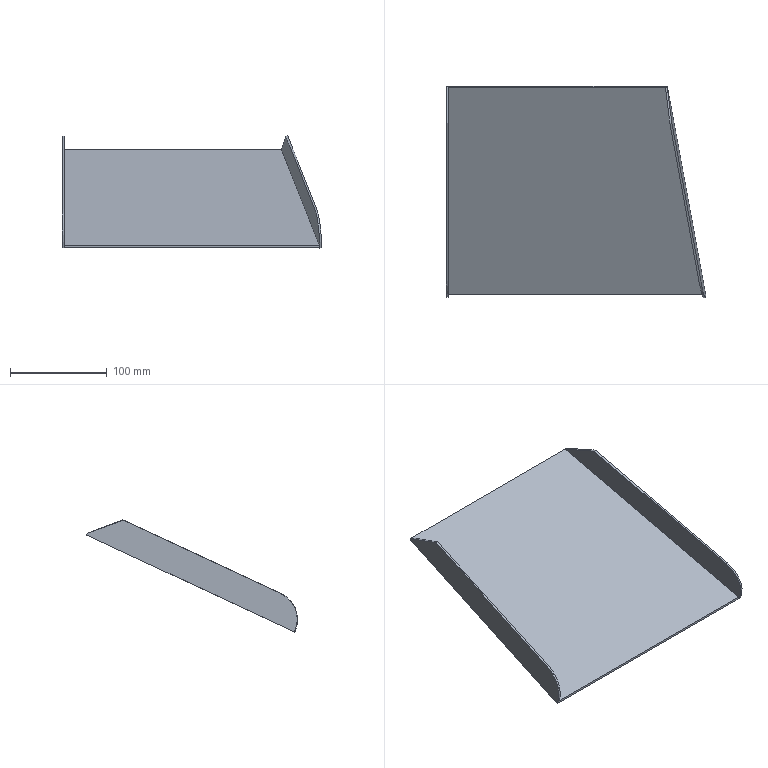Part | NX | features solid 2 | 1 solid | 14 faces | box 267.814 x 218.199 x 115.938 mm | volume 140586 mm3 | plane 11 | cylinder 2 | spline 1 | commonest cylinder face diameters 60 x2
STEP:
#1=CARTESIAN_POINT('',(712.,-840.,-299.582));
#2=VERTEX_POINT('',#1);
#3=CARTESIAN_POINT('',(975.787,-840.,-299.582));
#4=VERTEX_POINT('',#3);
#5=CARTESIAN_POINT('',(-476.248,-840.,-299.582));
#6=DIRECTION('',(1.,0.,0.));
#7=VECTOR('',#6,1000.);
#8=LINE('',#5,#7);
#9=EDGE_CURVE('',#2,#4,#8,.T.);
#10=ORIENTED_EDGE('',*,*,#9,.T.);
#11=CARTESIAN_POINT('',(975.631,-840.,-297.376));
#12=VERTEX_POINT('',#11);
#13=CARTESIAN_POINT('',(998.098,-840.,-616.062));
#14=DIRECTION('',(-0.07032,0.,0.9975));
#15=VECTOR('',#14,1000.);
#16=LINE('',#13,#15);
#17=EDGE_CURVE('',#4,#12,#16,.T.);
#18=ORIENTED_EDGE('',*,*,#17,.T.);
#19=CARTESIAN_POINT('',(712.,-840.,-297.376));
#20=VERTEX_POINT('',#19);
#21=CARTESIAN_POINT('',(-476.248,-840.,-297.376));
#22=DIRECTION('',(1.,0.,0.));
#23=VECTOR('',#22,1000.);
#24=LINE('',#21,#23);
#25=EDGE_CURVE('',#20,#12,#24,.T.);
#26=ORIENTED_EDGE('',*,*,#25,.F.);
#27=CARTESIAN_POINT('',(712.,-840.,-720.));
#28=DIRECTION('',(0.,0.,1.));
#29=VECTOR('',#28,1000.);
#30=LINE('',#27,#29);
#31=EDGE_CURVE('',#2,#20,#30,.T.);
#32=ORIENTED_EDGE('',*,*,#31,.F.);
#33=EDGE_LOOP('',(#10,#18,#26,#32));
#34=FACE_BOUND('',#33,.T.);
#35=CARTESIAN_POINT('',(-476.248,-840.,-720.));
#36=DIRECTION('',(0.,1.,0.));
#37=DIRECTION('',(-1.,0.,0.));
#38=AXIS2_PLACEMENT_3D('',#35,#36,#37);
#39=PLANE('',#38);
#40=ADVANCED_FACE('',(#34),#39,.F.);
#41=CARTESIAN_POINT('',(936.259,-626.089,-197.627));
#42=VERTEX_POINT('',#41);
#43=CARTESIAN_POINT('',(882.666,-334.91,-61.848));
#44=DIRECTION('',(0.1645,-0.894,-0.4169));
#45=VECTOR('',#44,1000.);
#46=LINE('',#43,#45);
#47=EDGE_CURVE('',#42,#12,#46,.T.);
#48=ORIENTED_EDGE('',*,*,#47,.F.);
#49=CARTESIAN_POINT('',(938.232,-625.791,-197.488));
#50=VERTEX_POINT('',#49);
#51=CARTESIAN_POINT('',(938.232,-625.791,-197.488));
#52=DIRECTION('',(0.9864,0.1491,0.06954));
#53=VECTOR('',#52,1000.);
#54=LINE('',#51,#53);
#55=EDGE_CURVE('',#42,#50,#54,.T.);
#56=ORIENTED_EDGE('',*,*,#55,.T.);
#57=CARTESIAN_POINT('',(712.,-626.036,-197.603));
#58=VERTEX_POINT('',#57);
#59=CARTESIAN_POINT('',(938.232,-625.791,-197.488));
#60=CARTESIAN_POINT('',(937.864,-625.821,-197.502));
#61=CARTESIAN_POINT('',(937.156,-625.853,-197.517));
#62=CARTESIAN_POINT('',(936.019,-625.866,-197.523));
#63=CARTESIAN_POINT('',(935.325,-625.866,-197.523));
#64=CARTESIAN_POINT('',(934.661,-625.862,-197.521));
#65=CARTESIAN_POINT('',(934.351,-625.859,-197.52));
#66=CARTESIAN_POINT('',(933.814,-625.856,-197.518));
#67=CARTESIAN_POINT('',(933.119,-625.851,-197.516));
#68=CARTESIAN_POINT('',(932.217,-625.847,-197.514));
#69=CARTESIAN_POINT('',(931.124,-625.843,-197.513));
#70=CARTESIAN_POINT('',(930.365,-625.841,-197.512));
#71=CARTESIAN_POINT('',(929.239,-625.839,-197.511));
#72=CARTESIAN_POINT('',(927.81,-625.837,-197.51));
#73=CARTESIAN_POINT('',(926.307,-625.836,-197.509));
#74=CARTESIAN_POINT('',(925.211,-625.836,-197.509));
#75=CARTESIAN_POINT('',(924.592,-625.836,-197.509));
#76=CARTESIAN_POINT('',(923.901,-625.836,-197.509));
#77=CARTESIAN_POINT('',(923.486,-625.836,-197.509));
#78=CARTESIAN_POINT('',(922.62,-625.837,-197.51));
#79=CARTESIAN_POINT('',(921.494,-625.838,-197.51));
#80=CARTESIAN_POINT('',(919.967,-625.841,-197.511));
#81=CARTESIAN_POINT('',(918.293,-625.844,-197.513));
#82=CARTESIAN_POINT('',(916.464,-625.847,-197.515));
#83=CARTESIAN_POINT('',(914.484,-625.852,-197.517));
#84=CARTESIAN_POINT('',(912.698,-625.856,-197.519));
#85=CARTESIAN_POINT('',(911.212,-625.86,-197.52));
#86=CARTESIAN_POINT('',(910.306,-625.862,-197.521));
#87=CARTESIAN_POINT('',(909.757,-625.864,-197.522));
#88=CARTESIAN_POINT('',(909.228,-625.865,-197.523));
#89=CARTESIAN_POINT('',(908.354,-625.867,-197.524));
#90=CARTESIAN_POINT('',(906.61,-625.872,-197.526));
#91=CARTESIAN_POINT('',(904.237,-625.878,-197.529));
#92=CARTESIAN_POINT('',(901.543,-625.885,-197.532));
#93=CARTESIAN_POINT('',(898.171,-625.894,-197.536));
#94=CARTESIAN_POINT('',(894.359,-625.903,-197.541));
#95=CARTESIAN_POINT('',(890.432,-625.913,-197.545));
#96=CARTESIAN_POINT('',(887.154,-625.921,-197.549));
#97=CARTESIAN_POINT('',(884.521,-625.928,-197.552));
#98=CARTESIAN_POINT('',(882.871,-625.932,-197.554));
#99=CARTESIAN_POINT('',(881.991,-625.933,-197.555));
#100=CARTESIAN_POINT('',(881.583,-625.934,-197.555));
#101=CARTESIAN_POINT('',(881.33,-625.935,-197.555));
#102=CARTESIAN_POINT('',(881.219,-625.935,-197.555));
#103=CARTESIAN_POINT('',(880.86,-625.936,-197.556));
#104=CARTESIAN_POINT('',(880.282,-625.937,-197.556));
#105=CARTESIAN_POINT('',(879.042,-625.939,-197.557));
#106=CARTESIAN_POINT('',(876.424,-625.942,-197.559));
#107=CARTESIAN_POINT('',(872.189,-625.947,-197.561));
#108=CARTESIAN_POINT('',(866.348,-625.953,-197.564));
#109=CARTESIAN_POINT('',(859.739,-625.957,-197.566));
#110=CARTESIAN_POINT('',(852.364,-625.961,-197.568));
#111=CARTESIAN_POINT('',(845.58,-625.964,-197.569));
#112=CARTESIAN_POINT('',(839.769,-625.966,-197.57));
#113=CARTESIAN_POINT('',(835.221,-625.967,-197.57));
#114=CARTESIAN_POINT('',(831.267,-625.968,-197.571));
#115=CARTESIAN_POINT('',(828.017,-625.969,-197.571));
#116=CARTESIAN_POINT('',(826.135,-625.969,-197.571));
#117=CARTESIAN_POINT('',(824.894,-625.969,-197.571));
#118=CARTESIAN_POINT('',(823.993,-625.97,-197.571));
#119=CARTESIAN_POINT('',(823.37,-625.97,-197.572));
#120=CARTESIAN_POINT('',(822.475,-625.97,-197.572));
#121=CARTESIAN_POINT('',(820.761,-625.97,-197.572));
#122=CARTESIAN_POINT('',(817.,-625.971,-197.572));
#123=CARTESIAN_POINT('',(811.23,-625.972,-197.573));
#124=CARTESIAN_POINT('',(804.273,-625.974,-197.574));
#125=CARTESIAN_POINT('',(794.975,-625.977,-197.575));
#126=CARTESIAN_POINT('',(783.298,-625.982,-197.577));
#127=CARTESIAN_POINT('',(769.206,-625.99,-197.581));
#128=CARTESIAN_POINT('',(755.031,-625.999,-197.585));
#129=CARTESIAN_POINT('',(736.021,-626.013,-197.592));
#130=CARTESIAN_POINT('',(721.641,-626.026,-197.598));
#131=CARTESIAN_POINT('',(712.,-626.036,-197.603));
#132=B_SPLINE_CURVE_WITH_KNOTS('',3,(#59,#60,#61,#62,#63,#64,#65,#66,#67,#68,#69,#70,#71,#72,#73,#74,#75,#76,#77,#78,#79,#80,#81,#82,#83,#84,#85,#86,#87,#88,#89,#90,#91,#92,#93,#94,#95,#96,#97,#98,#99,#100,#101,#102,#103,#104,#105,#106,#107,#108,#109,#110,#111,#112,#113,#114,#115,#116,#117,#118,#119,#120,#121,#122,#123,#124,#125,#126,#127,#128,#129,#130,#131),.UNSPECIFIED.,.F.,.F.,(4,1,1,1,1,1,1,1,1,1,1,1,1,1,1,1,1,1,1,1,1,1,1,1,1,1,1,1,1,1,1,1,1,1,1,1,1,1,1,1,1,1,1,1,1,1,1,1,1,1,1,1,1,1,1,1,1,1,1,1,1,1,1,1,1,1,1,1,1,1,4),(0.,0.007746,0.01162,0.01355,0.01549,0.01743,0.01936,0.02324,0.02711,0.03098,0.03486,0.03873,0.04647,0.05422,0.05809,0.06003,0.06196,0.06584,0.06971,0.07746,0.0852,0.09295,0.1007,0.1084,0.1162,0.1201,0.1239,0.1249,0.1259,0.1278,0.1317,0.1394,0.1472,0.1549,0.1704,0.1859,0.2014,0.2169,0.2324,0.2401,0.244,0.2479,0.2498,0.2517,0.2556,0.2633,0.2788,0.3098,0.3408,0.3718,0.4028,0.4338,0.4492,0.4647,0.4802,0.488,0.4957,0.4977,0.4996,0.5035,0.5073,0.5112,0.5267,0.5577,0.5887,0.6196,0.6816,0.7436,0.8055,0.8675,0.9914),.UNSPECIFIED.);
#133=EDGE_CURVE('',#58,#50,#132,.F.);
#134=ORIENTED_EDGE('',*,*,#133,.F.);
#135=CARTESIAN_POINT('',(712.,-651.161,-209.318));
#136=DIRECTION('',(0.,-0.9063,-0.4226));
#137=VECTOR('',#136,1000.);
#138=LINE('',#135,#137);
#139=EDGE_CURVE('',#58,#20,#138,.T.);
#140=ORIENTED_EDGE('',*,*,#139,.T.);
#141=ORIENTED_EDGE('',*,*,#25,.T.);
#142=EDGE_LOOP('',(#48,#56,#134,#140,#141));
#143=FACE_BOUND('',#142,.T.);
#144=CARTESIAN_POINT('',(-1209.175,-651.161,-209.318));
#145=DIRECTION('',(0.,-0.4226,0.9063));
#146=DIRECTION('',(1.,0.,0.));
#147=AXIS2_PLACEMENT_3D('',#144,#145,#146);
#148=PLANE('',#147);
#149=ADVANCED_FACE('',(#143),#148,.T.);
#150=CARTESIAN_POINT('',(972.878,-825.86,-259.887));
#151=VERTEX_POINT('',#150);
#152=CARTESIAN_POINT('',(977.814,-840.,-299.582));
#153=VERTEX_POINT('',#152);
#154=CARTESIAN_POINT('',(972.878,-813.181,-287.077));
#155=DIRECTION('',(-0.9864,-0.1491,-0.06954));
#156=DIRECTION('',(0.1495,-0.9888,0.));
#157=AXIS2_PLACEMENT_3D('',#154,#155,#156);
#158=CIRCLE('',#157,30.);
#159=EDGE_CURVE('',#151,#153,#158,.F.);
#160=ORIENTED_EDGE('',*,*,#159,.T.);
#161=CARTESIAN_POINT('',(938.232,-624.945,-199.301));
#162=VERTEX_POINT('',#161);
#163=CARTESIAN_POINT('',(884.639,-333.767,-63.522));
#164=DIRECTION('',(0.1645,-0.894,-0.4169));
#165=VECTOR('',#164,1000.);
#166=LINE('',#163,#165);
#167=EDGE_CURVE('',#162,#153,#166,.T.);
#168=ORIENTED_EDGE('',*,*,#167,.F.);
#169=CARTESIAN_POINT('',(938.232,-624.945,-199.301));
#170=CARTESIAN_POINT('',(938.232,-625.227,-198.696));
#171=CARTESIAN_POINT('',(938.232,-625.509,-198.092));
#172=CARTESIAN_POINT('',(938.232,-625.791,-197.488));
#173=B_SPLINE_CURVE_WITH_KNOTS('',3,(#169,#170,#171,#172),.UNSPECIFIED.,.F.,.F.,(4,4),(0.,1.),.UNSPECIFIED.);
#174=EDGE_CURVE('',#50,#162,#173,.F.);
#175=ORIENTED_EDGE('',*,*,#174,.F.);
#176=CARTESIAN_POINT('',(942.839,-662.655,-183.783));
#177=VERTEX_POINT('',#176);
#178=CARTESIAN_POINT('',(942.839,-662.655,-183.783));
#179=DIRECTION('',(-0.1163,0.931,-0.3461));
#180=VECTOR('',#179,1000.);
#181=LINE('',#178,#180);
#182=EDGE_CURVE('',#50,#177,#181,.F.);
#183=ORIENTED_EDGE('',*,*,#182,.T.);
#184=CARTESIAN_POINT('',(938.232,-637.624,-172.111));
#185=DIRECTION('',(0.1645,-0.894,-0.4169));
#186=VECTOR('',#185,1000.);
#187=LINE('',#184,#186);
#188=EDGE_CURVE('',#177,#151,#187,.T.);
#189=ORIENTED_EDGE('',*,*,#188,.T.);
#190=EDGE_LOOP('',(#160,#168,#175,#183,#189));
#191=FACE_BOUND('',#190,.T.);
#192=CARTESIAN_POINT('',(884.639,-334.612,-61.709));
#193=DIRECTION('',(0.9864,0.1491,0.06954));
#194=DIRECTION('',(-0.1495,0.9888,0.));
#195=AXIS2_PLACEMENT_3D('',#192,#193,#194);
#196=PLANE('',#195);
#197=ADVANCED_FACE('',(#191),#196,.T.);
#198=CARTESIAN_POINT('',(710.,-625.193,-199.416));
#199=VERTEX_POINT('',#198);
#200=CARTESIAN_POINT('',(938.232,-624.945,-199.301));
#201=CARTESIAN_POINT('',(937.861,-624.976,-199.315));
#202=CARTESIAN_POINT('',(937.146,-625.008,-199.33));
#203=CARTESIAN_POINT('',(935.994,-625.021,-199.336));
#204=CARTESIAN_POINT('',(935.293,-625.021,-199.336));
#205=CARTESIAN_POINT('',(934.612,-625.017,-199.334));
#206=CARTESIAN_POINT('',(934.327,-625.014,-199.333));
#207=CARTESIAN_POINT('',(933.775,-625.01,-199.331));
#208=CARTESIAN_POINT('',(933.074,-625.006,-199.329));
#209=CARTESIAN_POINT('',(932.161,-625.002,-199.327));
#210=CARTESIAN_POINT('',(931.043,-624.998,-199.325));
#211=CARTESIAN_POINT('',(930.308,-624.996,-199.324));
#212=CARTESIAN_POINT('',(929.159,-624.994,-199.323));
#213=CARTESIAN_POINT('',(928.01,-624.992,-199.322));
#214=CARTESIAN_POINT('',(926.804,-624.991,-199.322));
#215=CARTESIAN_POINT('',(925.885,-624.99,-199.322));
#216=CARTESIAN_POINT('',(925.087,-624.99,-199.322));
#217=CARTESIAN_POINT('',(924.471,-624.991,-199.322));
#218=CARTESIAN_POINT('',(923.915,-624.991,-199.322));
#219=CARTESIAN_POINT('',(923.692,-624.991,-199.322));
#220=CARTESIAN_POINT('',(923.263,-624.991,-199.322));
#221=CARTESIAN_POINT('',(922.533,-624.992,-199.322));
#222=CARTESIAN_POINT('',(921.363,-624.993,-199.323));
#223=CARTESIAN_POINT('',(919.816,-624.996,-199.324));
#224=CARTESIAN_POINT('',(918.111,-624.999,-199.326));
#225=CARTESIAN_POINT('',(916.249,-625.003,-199.327));
#226=CARTESIAN_POINT('',(914.234,-625.007,-199.33));
#227=CARTESIAN_POINT('',(912.417,-625.012,-199.332));
#228=CARTESIAN_POINT('',(911.093,-625.015,-199.333));
#229=CARTESIAN_POINT('',(910.291,-625.017,-199.334));
#230=CARTESIAN_POINT('',(909.755,-625.018,-199.335));
#231=CARTESIAN_POINT('',(908.92,-625.021,-199.336));
#232=CARTESIAN_POINT('',(907.928,-625.023,-199.337));
#233=CARTESIAN_POINT('',(906.178,-625.028,-199.339));
#234=CARTESIAN_POINT('',(903.808,-625.034,-199.342));
#235=CARTESIAN_POINT('',(901.116,-625.041,-199.345));
#236=CARTESIAN_POINT('',(897.752,-625.049,-199.349));
#237=CARTESIAN_POINT('',(893.956,-625.059,-199.354));
#238=CARTESIAN_POINT('',(890.061,-625.069,-199.358));
#239=CARTESIAN_POINT('',(886.824,-625.077,-199.362));
#240=CARTESIAN_POINT('',(884.675,-625.082,-199.364));
#241=CARTESIAN_POINT('',(883.287,-625.085,-199.366));
#242=CARTESIAN_POINT('',(882.405,-625.087,-199.367));
#243=CARTESIAN_POINT('',(881.827,-625.089,-199.367));
#244=CARTESIAN_POINT('',(881.401,-625.089,-199.368));
#245=CARTESIAN_POINT('',(881.251,-625.09,-199.368));
#246=CARTESIAN_POINT('',(880.651,-625.091,-199.368));
#247=CARTESIAN_POINT('',(879.987,-625.092,-199.369));
#248=CARTESIAN_POINT('',(878.713,-625.094,-199.37));
#249=CARTESIAN_POINT('',(876.807,-625.096,-199.371));
#250=CARTESIAN_POINT('',(874.309,-625.1,-199.373));
#251=CARTESIAN_POINT('',(870.725,-625.103,-199.374));
#252=CARTESIAN_POINT('',(865.755,-625.108,-199.376));
#253=CARTESIAN_POINT('',(859.012,-625.113,-199.379));
#254=CARTESIAN_POINT('',(851.49,-625.117,-199.381));
#255=CARTESIAN_POINT('',(844.572,-625.119,-199.382));
#256=CARTESIAN_POINT('',(838.648,-625.121,-199.383));
#257=CARTESIAN_POINT('',(834.783,-625.122,-199.383));
#258=CARTESIAN_POINT('',(831.594,-625.123,-199.383));
#259=CARTESIAN_POINT('',(829.151,-625.123,-199.384));
#260=CARTESIAN_POINT('',(827.085,-625.124,-199.384));
#261=CARTESIAN_POINT('',(825.596,-625.124,-199.384));
#262=CARTESIAN_POINT('',(824.772,-625.124,-199.384));
#263=CARTESIAN_POINT('',(824.058,-625.124,-199.384));
#264=CARTESIAN_POINT('',(823.697,-625.124,-199.384));
#265=CARTESIAN_POINT('',(823.092,-625.124,-199.384));
#266=CARTESIAN_POINT('',(822.091,-625.125,-199.384));
#267=CARTESIAN_POINT('',(820.63,-625.125,-199.384));
#268=CARTESIAN_POINT('',(818.888,-625.125,-199.385));
#269=CARTESIAN_POINT('',(816.559,-625.126,-199.385));
#270=CARTESIAN_POINT('',(813.647,-625.126,-199.385));
#271=CARTESIAN_POINT('',(808.978,-625.127,-199.386));
#272=CARTESIAN_POINT('',(803.13,-625.129,-199.386));
#273=CARTESIAN_POINT('',(796.092,-625.132,-199.388));
#274=CARTESIAN_POINT('',(789.033,-625.135,-199.389));
#275=CARTESIAN_POINT('',(779.592,-625.139,-199.391));
#276=CARTESIAN_POINT('',(767.74,-625.146,-199.394));
#277=CARTESIAN_POINT('',(753.434,-625.155,-199.398));
#278=CARTESIAN_POINT('',(734.247,-625.17,-199.405));
#279=CARTESIAN_POINT('',(719.732,-625.183,-199.412));
#280=CARTESIAN_POINT('',(710.,-625.193,-199.416));
#281=B_SPLINE_CURVE_WITH_KNOTS('',3,(#200,#201,#202,#203,#204,#205,#206,#207,#208,#209,#210,#211,#212,#213,#214,#215,#216,#217,#218,#219,#220,#221,#222,#223,#224,#225,#226,#227,#228,#229,#230,#231,#232,#233,#234,#235,#236,#237,#238,#239,#240,#241,#242,#243,#244,#245,#246,#247,#248,#249,#250,#251,#252,#253,#254,#255,#256,#257,#258,#259,#260,#261,#262,#263,#264,#265,#266,#267,#268,#269,#270,#271,#272,#273,#274,#275,#276,#277,#278,#279,#280),.UNSPECIFIED.,.F.,.F.,(4,1,1,1,1,1,1,1,1,1,1,1,1,1,1,1,1,1,1,1,1,1,1,1,1,1,1,1,1,1,1,1,1,1,1,1,1,1,1,1,1,1,1,1,1,1,1,1,1,1,1,1,1,1,1,1,1,1,1,1,1,1,1,1,1,1,1,1,1,1,1,1,1,1,1,1,1,1,4),(0.,0.007812,0.01172,0.01367,0.01562,0.01758,0.01953,0.02344,0.02734,0.03125,0.03516,0.03906,0.04688,0.05078,0.05469,0.05859,0.06055,0.0625,0.06445,0.06641,0.07031,0.07812,0.08594,0.09375,0.1016,0.1094,0.1172,0.1211,0.123,0.125,0.127,0.1289,0.1328,0.1406,0.1484,0.1562,0.1719,0.1875,0.2031,0.2188,0.2266,0.2344,0.2422,0.2461,0.25,0.2539,0.2578,0.2656,0.2812,0.2969,0.3125,0.3438,0.375,0.4062,0.4375,0.4531,0.4688,0.4766,0.4844,0.4922,0.4961,0.498,0.5,0.502,0.5039,0.5078,0.5156,0.5234,0.5312,0.5469,0.5625,0.5938,0.625,0.6562,0.6875,0.75,0.8125,0.875,1.),.UNSPECIFIED.);
#282=EDGE_CURVE('',#199,#162,#281,.F.);
#283=ORIENTED_EDGE('',*,*,#282,.F.);
#284=CARTESIAN_POINT('',(710.,-626.038,-197.604));
#285=VERTEX_POINT('',#284);
#286=CARTESIAN_POINT('',(710.,-626.038,-197.604));
#287=CARTESIAN_POINT('',(710.,-625.757,-198.208));
#288=CARTESIAN_POINT('',(710.,-625.475,-198.812));
#289=CARTESIAN_POINT('',(710.,-625.193,-199.416));
#290=B_SPLINE_CURVE_WITH_KNOTS('',3,(#286,#287,#288,#289),.UNSPECIFIED.,.F.,.F.,(4,4),(0.,1.),.UNSPECIFIED.);
#291=EDGE_CURVE('',#285,#199,#290,.T.);
#292=ORIENTED_EDGE('',*,*,#291,.F.);
#293=CARTESIAN_POINT('',(712.,-626.038,-197.604));
#294=CARTESIAN_POINT('',(711.333,-626.038,-197.604));
#295=CARTESIAN_POINT('',(710.667,-626.038,-197.604));
#296=CARTESIAN_POINT('',(710.,-626.038,-197.604));
#297=B_SPLINE_CURVE_WITH_KNOTS('',3,(#293,#294,#295,#296),.UNSPECIFIED.,.F.,.F.,(4,4),(0.,1.),.UNSPECIFIED.);
#298=EDGE_CURVE('',#285,#58,#297,.F.);
#299=ORIENTED_EDGE('',*,*,#298,.T.);
#300=ORIENTED_EDGE('',*,*,#133,.T.);
#301=ORIENTED_EDGE('',*,*,#174,.T.);
#302=EDGE_LOOP('',(#283,#292,#299,#300,#301));
#303=FACE_BOUND('',#302,.T.);
#304=CARTESIAN_POINT('',(938.232,-625.791,-197.488));
#305=CARTESIAN_POINT('',(938.232,-624.945,-199.301));
#306=CARTESIAN_POINT('',(937.861,-625.821,-197.502));
#307=CARTESIAN_POINT('',(937.861,-624.976,-199.315));
#308=CARTESIAN_POINT('',(937.146,-625.853,-197.517));
#309=CARTESIAN_POINT('',(937.146,-625.008,-199.33));
#310=CARTESIAN_POINT('',(935.994,-625.866,-197.523));
#311=CARTESIAN_POINT('',(935.994,-625.021,-199.336));
#312=CARTESIAN_POINT('',(935.293,-625.866,-197.523));
#313=CARTESIAN_POINT('',(935.293,-625.021,-199.336));
#314=CARTESIAN_POINT('',(934.612,-625.862,-197.521));
#315=CARTESIAN_POINT('',(934.612,-625.017,-199.334));
#316=CARTESIAN_POINT('',(934.327,-625.859,-197.52));
#317=CARTESIAN_POINT('',(934.327,-625.014,-199.333));
#318=CARTESIAN_POINT('',(933.775,-625.855,-197.518));
#319=CARTESIAN_POINT('',(933.775,-625.01,-199.331));
#320=CARTESIAN_POINT('',(933.074,-625.851,-197.516));
#321=CARTESIAN_POINT('',(933.074,-625.006,-199.329));
#322=CARTESIAN_POINT('',(932.161,-625.847,-197.514));
#323=CARTESIAN_POINT('',(932.161,-625.002,-199.327));
#324=CARTESIAN_POINT('',(931.043,-625.843,-197.513));
#325=CARTESIAN_POINT('',(931.043,-624.998,-199.325));
#326=CARTESIAN_POINT('',(930.308,-625.841,-197.512));
#327=CARTESIAN_POINT('',(930.308,-624.996,-199.324));
#328=CARTESIAN_POINT('',(929.159,-625.839,-197.511));
#329=CARTESIAN_POINT('',(929.159,-624.994,-199.323));
#330=CARTESIAN_POINT('',(928.01,-625.837,-197.51));
#331=CARTESIAN_POINT('',(928.01,-624.992,-199.322));
#332=CARTESIAN_POINT('',(926.804,-625.836,-197.509));
#333=CARTESIAN_POINT('',(926.804,-624.991,-199.322));
#334=CARTESIAN_POINT('',(925.885,-625.836,-197.509));
#335=CARTESIAN_POINT('',(925.885,-624.99,-199.322));
#336=CARTESIAN_POINT('',(925.087,-625.836,-197.509));
#337=CARTESIAN_POINT('',(925.087,-624.99,-199.322));
#338=CARTESIAN_POINT('',(924.471,-625.836,-197.509));
#339=CARTESIAN_POINT('',(924.471,-624.991,-199.322));
#340=CARTESIAN_POINT('',(923.915,-625.836,-197.509));
#341=CARTESIAN_POINT('',(923.915,-624.991,-199.322));
#342=CARTESIAN_POINT('',(923.692,-625.836,-197.509));
#343=CARTESIAN_POINT('',(923.692,-624.991,-199.322));
#344=CARTESIAN_POINT('',(923.263,-625.837,-197.509));
#345=CARTESIAN_POINT('',(923.263,-624.991,-199.322));
#346=CARTESIAN_POINT('',(922.533,-625.837,-197.51));
#347=CARTESIAN_POINT('',(922.533,-624.992,-199.322));
#348=CARTESIAN_POINT('',(921.363,-625.839,-197.51));
#349=CARTESIAN_POINT('',(921.363,-624.993,-199.323));
#350=CARTESIAN_POINT('',(919.816,-625.841,-197.512));
#351=CARTESIAN_POINT('',(919.816,-624.996,-199.324));
#352=CARTESIAN_POINT('',(918.111,-625.844,-197.513));
#353=CARTESIAN_POINT('',(918.111,-624.999,-199.326));
#354=CARTESIAN_POINT('',(916.249,-625.848,-197.515));
#355=CARTESIAN_POINT('',(916.249,-625.003,-199.327));
#356=CARTESIAN_POINT('',(914.234,-625.852,-197.517));
#357=CARTESIAN_POINT('',(914.234,-625.007,-199.33));
#358=CARTESIAN_POINT('',(912.417,-625.857,-197.519));
#359=CARTESIAN_POINT('',(912.417,-625.012,-199.332));
#360=CARTESIAN_POINT('',(911.093,-625.86,-197.52));
#361=CARTESIAN_POINT('',(911.093,-625.015,-199.333));
#362=CARTESIAN_POINT('',(910.291,-625.862,-197.521));
#363=CARTESIAN_POINT('',(910.291,-625.017,-199.334));
#364=CARTESIAN_POINT('',(909.755,-625.864,-197.522));
#365=CARTESIAN_POINT('',(909.755,-625.018,-199.335));
#366=CARTESIAN_POINT('',(908.92,-625.866,-197.523));
#367=CARTESIAN_POINT('',(908.92,-625.021,-199.336));
#368=CARTESIAN_POINT('',(907.928,-625.868,-197.524));
#369=CARTESIAN_POINT('',(907.928,-625.023,-199.337));
#370=CARTESIAN_POINT('',(906.178,-625.873,-197.526));
#371=CARTESIAN_POINT('',(906.178,-625.028,-199.339));
#372=CARTESIAN_POINT('',(903.808,-625.879,-197.529));
#373=CARTESIAN_POINT('',(903.808,-625.034,-199.342));
#374=CARTESIAN_POINT('',(901.116,-625.886,-197.533));
#375=CARTESIAN_POINT('',(901.116,-625.041,-199.345));
#376=CARTESIAN_POINT('',(897.752,-625.895,-197.537));
#377=CARTESIAN_POINT('',(897.752,-625.049,-199.349));
#378=CARTESIAN_POINT('',(893.956,-625.904,-197.541));
#379=CARTESIAN_POINT('',(893.956,-625.059,-199.354));
#380=CARTESIAN_POINT('',(890.061,-625.914,-197.546));
#381=CARTESIAN_POINT('',(890.061,-625.069,-199.358));
#382=CARTESIAN_POINT('',(886.824,-625.922,-197.549));
#383=CARTESIAN_POINT('',(886.824,-625.077,-199.362));
#384=CARTESIAN_POINT('',(884.675,-625.927,-197.552));
#385=CARTESIAN_POINT('',(884.675,-625.082,-199.364));
#386=CARTESIAN_POINT('',(883.287,-625.931,-197.553));
#387=CARTESIAN_POINT('',(883.287,-625.085,-199.366));
#388=CARTESIAN_POINT('',(882.405,-625.933,-197.554));
#389=CARTESIAN_POINT('',(882.405,-625.087,-199.367));
#390=CARTESIAN_POINT('',(881.827,-625.934,-197.555));
#391=CARTESIAN_POINT('',(881.827,-625.089,-199.367));
#392=CARTESIAN_POINT('',(881.401,-625.935,-197.555));
#393=CARTESIAN_POINT('',(881.401,-625.089,-199.368));
#394=CARTESIAN_POINT('',(881.251,-625.935,-197.555));
#395=CARTESIAN_POINT('',(881.251,-625.09,-199.368));
#396=CARTESIAN_POINT('',(880.651,-625.936,-197.556));
#397=CARTESIAN_POINT('',(880.651,-625.091,-199.368));
#398=CARTESIAN_POINT('',(879.987,-625.937,-197.556));
#399=CARTESIAN_POINT('',(879.987,-625.092,-199.369));
#400=CARTESIAN_POINT('',(878.713,-625.939,-197.557));
#401=CARTESIAN_POINT('',(878.713,-625.094,-199.37));
#402=CARTESIAN_POINT('',(876.807,-625.942,-197.559));
#403=CARTESIAN_POINT('',(876.807,-625.096,-199.371));
#404=CARTESIAN_POINT('',(874.309,-625.945,-197.56));
#405=CARTESIAN_POINT('',(874.309,-625.1,-199.373));
#406=CARTESIAN_POINT('',(870.725,-625.949,-197.562));
#407=CARTESIAN_POINT('',(870.725,-625.103,-199.374));
#408=CARTESIAN_POINT('',(865.755,-625.953,-197.564));
#409=CARTESIAN_POINT('',(865.755,-625.108,-199.376));
#410=CARTESIAN_POINT('',(859.012,-625.958,-197.566));
#411=CARTESIAN_POINT('',(859.012,-625.113,-199.379));
#412=CARTESIAN_POINT('',(851.49,-625.962,-197.568));
#413=CARTESIAN_POINT('',(851.49,-625.117,-199.381));
#414=CARTESIAN_POINT('',(844.572,-625.965,-197.569));
#415=CARTESIAN_POINT('',(844.572,-625.119,-199.382));
#416=CARTESIAN_POINT('',(838.648,-625.966,-197.57));
#417=CARTESIAN_POINT('',(838.648,-625.121,-199.383));
#418=CARTESIAN_POINT('',(834.783,-625.967,-197.571));
#419=CARTESIAN_POINT('',(834.783,-625.122,-199.383));
#420=CARTESIAN_POINT('',(831.594,-625.968,-197.571));
#421=CARTESIAN_POINT('',(831.594,-625.123,-199.383));
#422=CARTESIAN_POINT('',(829.151,-625.969,-197.571));
#423=CARTESIAN_POINT('',(829.151,-625.123,-199.384));
#424=CARTESIAN_POINT('',(827.085,-625.969,-197.571));
#425=CARTESIAN_POINT('',(827.085,-625.124,-199.384));
#426=CARTESIAN_POINT('',(825.596,-625.969,-197.571));
#427=CARTESIAN_POINT('',(825.596,-625.124,-199.384));
#428=CARTESIAN_POINT('',(824.772,-625.969,-197.571));
#429=CARTESIAN_POINT('',(824.772,-625.124,-199.384));
#430=CARTESIAN_POINT('',(824.058,-625.97,-197.571));
#431=CARTESIAN_POINT('',(824.058,-625.124,-199.384));
#432=CARTESIAN_POINT('',(823.697,-625.97,-197.572));
#433=CARTESIAN_POINT('',(823.697,-625.124,-199.384));
#434=CARTESIAN_POINT('',(823.092,-625.97,-197.572));
#435=CARTESIAN_POINT('',(823.092,-625.124,-199.384));
#436=CARTESIAN_POINT('',(822.091,-625.97,-197.572));
#437=CARTESIAN_POINT('',(822.091,-625.125,-199.384));
#438=CARTESIAN_POINT('',(820.63,-625.97,-197.572));
#439=CARTESIAN_POINT('',(820.63,-625.125,-199.384));
#440=CARTESIAN_POINT('',(818.888,-625.97,-197.572));
#441=CARTESIAN_POINT('',(818.888,-625.125,-199.385));
#442=CARTESIAN_POINT('',(816.559,-625.971,-197.572));
#443=CARTESIAN_POINT('',(816.559,-625.126,-199.385));
#444=CARTESIAN_POINT('',(813.647,-625.972,-197.572));
#445=CARTESIAN_POINT('',(813.647,-625.126,-199.385));
#446=CARTESIAN_POINT('',(808.978,-625.973,-197.573));
#447=CARTESIAN_POINT('',(808.978,-625.127,-199.386));
#448=CARTESIAN_POINT('',(803.13,-625.974,-197.574));
#449=CARTESIAN_POINT('',(803.13,-625.129,-199.386));
#450=CARTESIAN_POINT('',(796.092,-625.977,-197.575));
#451=CARTESIAN_POINT('',(796.092,-625.132,-199.388));
#452=CARTESIAN_POINT('',(789.033,-625.98,-197.576));
#453=CARTESIAN_POINT('',(789.033,-625.135,-199.389));
#454=CARTESIAN_POINT('',(760.712,-625.993,-197.582));
#455=CARTESIAN_POINT('',(760.712,-625.148,-199.395));
#456=CARTESIAN_POINT('',(734.331,-626.013,-197.592));
#457=CARTESIAN_POINT('',(734.331,-625.168,-199.404));
#458=CARTESIAN_POINT('',(710.,-626.038,-197.604));
#459=CARTESIAN_POINT('',(710.,-625.193,-199.416));
#460=B_SPLINE_SURFACE_WITH_KNOTS('',3,1,((#304,#305),(#306,#307),(#308,#309),(#310,#311),(#312,#313),(#314,#315),(#316,#317),(#318,#319),(#320,#321),(#322,#323),(#324,#325),(#326,#327),(#328,#329),(#330,#331),(#332,#333),(#334,#335),(#336,#337),(#338,#339),(#340,#341),(#342,#343),(#344,#345),(#346,#347),(#348,#349),(#350,#351),(#352,#353),(#354,#355),(#356,#357),(#358,#359),(#360,#361),(#362,#363),(#364,#365),(#366,#367),(#368,#369),(#370,#371),(#372,#373),(#374,#375),(#376,#377),(#378,#379),(#380,#381),(#382,#383),(#384,#385),(#386,#387),(#388,#389),(#390,#391),(#392,#393),(#394,#395),(#396,#397),(#398,#399),(#400,#401),(#402,#403),(#404,#405),(#406,#407),(#408,#409),(#410,#411),(#412,#413),(#414,#415),(#416,#417),(#418,#419),(#420,#421),(#422,#423),(#424,#425),(#426,#427),(#428,#429),(#430,#431),(#432,#433),(#434,#435),(#436,#437),(#438,#439),(#440,#441),(#442,#443),(#444,#445),(#446,#447),(#448,#449),(#450,#451),(#452,#453),(#454,#455),(#456,#457),(#458,#459)),.UNSPECIFIED.,.F.,.F.,.F.,(4,1,1,1,1,1,1,1,1,1,1,1,1,1,1,1,1,1,1,1,1,1,1,1,1,1,1,1,1,1,1,1,1,1,1,1,1,1,1,1,1,1,1,1,1,1,1,1,1,1,1,1,1,1,1,1,1,1,1,1,1,1,1,1,1,1,1,1,1,1,1,1,1,1,1,4),(2,2),(0.,0.007812,0.01172,0.01367,0.01562,0.01758,0.01953,0.02344,0.02734,0.03125,0.03516,0.03906,0.04688,0.05078,0.05469,0.05859,0.06055,0.0625,0.06445,0.06641,0.07031,0.07812,0.08594,0.09375,0.1016,0.1094,0.1172,0.1211,0.123,0.125,0.127,0.1289,0.1328,0.1406,0.1484,0.1562,0.1719,0.1875,0.2031,0.2188,0.2266,0.2344,0.2422,0.2461,0.25,0.2539,0.2578,0.2656,0.2812,0.2969,0.3125,0.3438,0.375,0.4062,0.4375,0.4531,0.4688,0.4766,0.4844,0.4922,0.4961,0.498,0.5,0.502,0.5039,0.5078,0.5156,0.5234,0.5312,0.5469,0.5625,0.5938,0.625,0.6562,0.6875,1.),(0.,1.),.UNSPECIFIED.);
#461=ADVANCED_FACE('',(#303),#460,.F.);
#462=CARTESIAN_POINT('',(710.,-840.,-299.582));
#463=VERTEX_POINT('',#462);
#464=CARTESIAN_POINT('',(710.,-650.315,-211.131));
#465=DIRECTION('',(0.,-0.9063,-0.4226));
#466=VECTOR('',#465,1000.);
#467=LINE('',#464,#466);
#468=EDGE_CURVE('',#199,#463,#467,.T.);
#469=ORIENTED_EDGE('',*,*,#468,.T.);
#470=CARTESIAN_POINT('',(710.,-825.489,-259.715));
#471=VERTEX_POINT('',#470);
#472=CARTESIAN_POINT('',(710.,-812.811,-286.904));
#473=DIRECTION('',(-1.,0.,0.));
#474=DIRECTION('',(0.,0.,1.));
#475=AXIS2_PLACEMENT_3D('',#472,#473,#474);
#476=CIRCLE('',#475,30.);
#477=EDGE_CURVE('',#463,#471,#476,.T.);
#478=ORIENTED_EDGE('',*,*,#477,.T.);
#479=CARTESIAN_POINT('',(710.,-663.248,-184.06));
#480=VERTEX_POINT('',#479);
#481=CARTESIAN_POINT('',(710.,-637.872,-172.227));
#482=DIRECTION('',(0.,-0.9063,-0.4226));
#483=VECTOR('',#482,1000.);
#484=LINE('',#481,#483);
#485=EDGE_CURVE('',#480,#471,#484,.T.);
#486=ORIENTED_EDGE('',*,*,#485,.F.);
#487=CARTESIAN_POINT('',(710.,-624.709,-198.087));
#488=DIRECTION('',(0.,-0.9397,0.342));
#489=VECTOR('',#488,1000.);
#490=LINE('',#487,#489);
#491=EDGE_CURVE('',#480,#285,#490,.F.);
#492=ORIENTED_EDGE('',*,*,#491,.T.);
#493=ORIENTED_EDGE('',*,*,#291,.T.);
#494=EDGE_LOOP('',(#469,#478,#486,#492,#493));
#495=FACE_BOUND('',#494,.T.);
#496=CARTESIAN_POINT('',(710.,-651.161,-209.318));
#497=DIRECTION('',(1.,0.,0.));
#498=DIRECTION('',(0.,1.,0.));
#499=AXIS2_PLACEMENT_3D('',#496,#497,#498);
#500=PLANE('',#499);
#501=ADVANCED_FACE('',(#495),#500,.F.);
#502=ORIENTED_EDGE('',*,*,#282,.T.);
#503=ORIENTED_EDGE('',*,*,#167,.T.);
#504=CARTESIAN_POINT('',(975.842,-840.298,-299.721));
#505=VERTEX_POINT('',#504);
#506=CARTESIAN_POINT('',(977.814,-840.,-299.582));
#507=DIRECTION('',(0.9864,0.1491,0.06954));
#508=VECTOR('',#507,1000.);
#509=LINE('',#506,#508);
#510=EDGE_CURVE('',#153,#505,#509,.F.);
#511=ORIENTED_EDGE('',*,*,#510,.T.);
#512=CARTESIAN_POINT('',(936.259,-625.244,-199.44));
#513=DIRECTION('',(0.1645,-0.894,-0.4169));
#514=VECTOR('',#513,1000.);
#515=LINE('',#512,#514);
#516=EDGE_CURVE('',#4,#505,#515,.T.);
#517=ORIENTED_EDGE('',*,*,#516,.F.);
#518=ORIENTED_EDGE('',*,*,#9,.F.);
#519=CARTESIAN_POINT('',(-476.248,-840.,-299.582));
#520=DIRECTION('',(1.,0.,0.));
#521=VECTOR('',#520,1000.);
#522=LINE('',#519,#521);
#523=EDGE_CURVE('',#463,#2,#522,.T.);
#524=ORIENTED_EDGE('',*,*,#523,.F.);
#525=ORIENTED_EDGE('',*,*,#468,.F.);
#526=EDGE_LOOP('',(#502,#503,#511,#517,#518,#524,#525));
#527=FACE_BOUND('',#526,.T.);
#528=CARTESIAN_POINT('',(-1209.175,-650.315,-211.131));
#529=DIRECTION('',(0.,-0.4226,0.9063));
#530=DIRECTION('',(1.,0.,0.));
#531=AXIS2_PLACEMENT_3D('',#528,#529,#530);
#532=PLANE('',#531);
#533=ADVANCED_FACE('',(#527),#532,.F.);
#534=CARTESIAN_POINT('',(712.,-825.489,-259.715));
#535=VERTEX_POINT('',#534);
#536=CARTESIAN_POINT('',(712.,-812.811,-286.904));
#537=DIRECTION('',(-1.,0.,0.));
#538=DIRECTION('',(0.,0.,1.));
#539=AXIS2_PLACEMENT_3D('',#536,#537,#538);
#540=CIRCLE('',#539,30.);
#541=EDGE_CURVE('',#535,#2,#540,.F.);
#542=ORIENTED_EDGE('',*,*,#541,.T.);
#543=ORIENTED_EDGE('',*,*,#31,.T.);
#544=ORIENTED_EDGE('',*,*,#139,.F.);
#545=CARTESIAN_POINT('',(712.,-663.248,-184.06));
#546=VERTEX_POINT('',#545);
#547=CARTESIAN_POINT('',(712.,-626.038,-197.604));
#548=DIRECTION('',(0.,0.9397,-0.342));
#549=VECTOR('',#548,1000.);
#550=LINE('',#547,#549);
#551=EDGE_CURVE('',#58,#546,#550,.F.);
#552=ORIENTED_EDGE('',*,*,#551,.T.);
#553=CARTESIAN_POINT('',(712.,-637.872,-172.227));
#554=DIRECTION('',(0.,-0.9063,-0.4226));
#555=VECTOR('',#554,1000.);
#556=LINE('',#553,#555);
#557=EDGE_CURVE('',#546,#535,#556,.T.);
#558=ORIENTED_EDGE('',*,*,#557,.T.);
#559=EDGE_LOOP('',(#542,#543,#544,#552,#558));
#560=FACE_BOUND('',#559,.T.);
#561=CARTESIAN_POINT('',(712.,-625.193,-199.416));
#562=DIRECTION('',(-1.,0.,0.));
#563=DIRECTION('',(0.,0.,1.));
#564=AXIS2_PLACEMENT_3D('',#561,#562,#563);
#565=PLANE('',#564);
#566=ADVANCED_FACE('',(#560),#565,.F.);
#567=ORIENTED_EDGE('',*,*,#485,.T.);
#568=CARTESIAN_POINT('',(710.,-825.489,-259.715));
#569=DIRECTION('',(1.,0.,0.));
#570=VECTOR('',#569,1000.);
#571=LINE('',#568,#570);
#572=EDGE_CURVE('',#471,#535,#571,.T.);
#573=ORIENTED_EDGE('',*,*,#572,.T.);
#574=ORIENTED_EDGE('',*,*,#557,.F.);
#575=CARTESIAN_POINT('',(710.,-663.248,-184.06));
#576=DIRECTION('',(1.,0.,0.));
#577=VECTOR('',#576,1000.);
#578=LINE('',#575,#577);
#579=EDGE_CURVE('',#546,#480,#578,.F.);
#580=ORIENTED_EDGE('',*,*,#579,.T.);
#581=EDGE_LOOP('',(#567,#573,#574,#580));
#582=FACE_BOUND('',#581,.T.);
#583=CARTESIAN_POINT('',(710.,-637.872,-172.227));
#584=DIRECTION('',(0.,0.4226,-0.9063));
#585=DIRECTION('',(0.,-0.9063,-0.4226));
#586=AXIS2_PLACEMENT_3D('',#583,#584,#585);
#587=PLANE('',#586);
#588=ADVANCED_FACE('',(#582),#587,.F.);
#589=ORIENTED_EDGE('',*,*,#491,.F.);
#590=ORIENTED_EDGE('',*,*,#579,.F.);
#591=ORIENTED_EDGE('',*,*,#551,.F.);
#592=ORIENTED_EDGE('',*,*,#298,.F.);
#593=EDGE_LOOP('',(#589,#590,#591,#592));
#594=FACE_BOUND('',#593,.T.);
#595=CARTESIAN_POINT('',(710.,-626.038,-197.604));
#596=DIRECTION('',(0.,-0.342,-0.9397));
#597=DIRECTION('',(0.,0.9397,-0.342));
#598=AXIS2_PLACEMENT_3D('',#595,#596,#597);
#599=PLANE('',#598);
#600=ADVANCED_FACE('',(#594),#599,.F.);
#601=ORIENTED_EDGE('',*,*,#477,.F.);
#602=ORIENTED_EDGE('',*,*,#523,.T.);
#603=ORIENTED_EDGE('',*,*,#541,.F.);
#604=ORIENTED_EDGE('',*,*,#572,.F.);
#605=EDGE_LOOP('',(#601,#602,#603,#604));
#606=FACE_BOUND('',#605,.T.);
#607=CARTESIAN_POINT('',(710.,-812.811,-286.904));
#608=DIRECTION('',(-1.,0.,0.));
#609=DIRECTION('',(0.,0.,1.));
#610=AXIS2_PLACEMENT_3D('',#607,#608,#609);
#611=CYLINDRICAL_SURFACE('',#610,30.);
#612=ADVANCED_FACE('',(#606),#611,.T.);
#613=ORIENTED_EDGE('',*,*,#17,.F.);
#614=ORIENTED_EDGE('',*,*,#516,.T.);
#615=CARTESIAN_POINT('',(970.906,-826.158,-260.026));
#616=VERTEX_POINT('',#615);
#617=CARTESIAN_POINT('',(970.906,-813.48,-287.216));
#618=DIRECTION('',(-0.9864,-0.1491,-0.06954));
#619=DIRECTION('',(0.1495,-0.9888,0.));
#620=AXIS2_PLACEMENT_3D('',#617,#618,#619);
#621=CIRCLE('',#620,30.);
#622=EDGE_CURVE('',#505,#616,#621,.T.);
#623=ORIENTED_EDGE('',*,*,#622,.T.);
#624=CARTESIAN_POINT('',(940.867,-662.953,-183.923));
#625=VERTEX_POINT('',#624);
#626=CARTESIAN_POINT('',(936.259,-637.922,-172.251));
#627=DIRECTION('',(0.1645,-0.894,-0.4169));
#628=VECTOR('',#627,1000.);
#629=LINE('',#626,#628);
#630=EDGE_CURVE('',#625,#616,#629,.T.);
#631=ORIENTED_EDGE('',*,*,#630,.F.);
#632=CARTESIAN_POINT('',(936.095,-624.772,-198.117));
#633=DIRECTION('',(0.1163,-0.931,0.3461));
#634=VECTOR('',#633,1000.);
#635=LINE('',#632,#634);
#636=EDGE_CURVE('',#625,#42,#635,.F.);
#637=ORIENTED_EDGE('',*,*,#636,.T.);
#638=ORIENTED_EDGE('',*,*,#47,.T.);
#639=EDGE_LOOP('',(#613,#614,#623,#631,#637,#638));
#640=FACE_BOUND('',#639,.T.);
#641=CARTESIAN_POINT('',(936.259,-625.244,-199.44));
#642=DIRECTION('',(-0.9864,-0.1491,-0.06954));
#643=DIRECTION('',(0.1495,-0.9888,0.));
#644=AXIS2_PLACEMENT_3D('',#641,#642,#643);
#645=PLANE('',#644);
#646=ADVANCED_FACE('',(#640),#645,.T.);
#647=ORIENTED_EDGE('',*,*,#630,.T.);
#648=CARTESIAN_POINT('',(972.878,-825.86,-259.887));
#649=DIRECTION('',(0.9864,0.1491,0.06954));
#650=VECTOR('',#649,1000.);
#651=LINE('',#648,#650);
#652=EDGE_CURVE('',#616,#151,#651,.T.);
#653=ORIENTED_EDGE('',*,*,#652,.T.);
#654=ORIENTED_EDGE('',*,*,#188,.F.);
#655=CARTESIAN_POINT('',(942.839,-662.655,-183.783));
#656=DIRECTION('',(-0.9864,-0.1491,-0.06954));
#657=VECTOR('',#656,1000.);
#658=LINE('',#655,#657);
#659=EDGE_CURVE('',#177,#625,#658,.T.);
#660=ORIENTED_EDGE('',*,*,#659,.T.);
#661=EDGE_LOOP('',(#647,#653,#654,#660));
#662=FACE_BOUND('',#661,.T.);
#663=CARTESIAN_POINT('',(938.232,-637.624,-172.111));
#664=DIRECTION('',(0.,0.4226,-0.9063));
#665=DIRECTION('',(0.1645,-0.894,-0.4169));
#666=AXIS2_PLACEMENT_3D('',#663,#664,#665);
#667=PLANE('',#666);
#668=ADVANCED_FACE('',(#662),#667,.F.);
#669=ORIENTED_EDGE('',*,*,#182,.F.);
#670=ORIENTED_EDGE('',*,*,#55,.F.);
#671=ORIENTED_EDGE('',*,*,#636,.F.);
#672=ORIENTED_EDGE('',*,*,#659,.F.);
#673=EDGE_LOOP('',(#669,#670,#671,#672));
#674=FACE_BOUND('',#673,.T.);
#675=CARTESIAN_POINT('',(942.839,-662.655,-183.783));
#676=DIRECTION('',(0.1163,-0.3333,-0.9356));
#677=DIRECTION('',(0.,0.942,-0.3356));
#678=AXIS2_PLACEMENT_3D('',#675,#676,#677);
#679=PLANE('',#678);
#680=ADVANCED_FACE('',(#674),#679,.F.);
#681=ORIENTED_EDGE('',*,*,#159,.F.);
#682=ORIENTED_EDGE('',*,*,#652,.F.);
#683=ORIENTED_EDGE('',*,*,#622,.F.);
#684=ORIENTED_EDGE('',*,*,#510,.F.);
#685=EDGE_LOOP('',(#681,#682,#683,#684));
#686=FACE_BOUND('',#685,.T.);
#687=CARTESIAN_POINT('',(972.878,-813.181,-287.077));
#688=DIRECTION('',(0.9864,0.1491,0.06954));
#689=DIRECTION('',(-0.1495,0.9888,0.));
#690=AXIS2_PLACEMENT_3D('',#687,#688,#689);
#691=CYLINDRICAL_SURFACE('',#690,30.);
#692=ADVANCED_FACE('',(#686),#691,.T.);
#693=CLOSED_SHELL('',(#40,#149,#197,#461,#501,#533,#566,#588,#600,#612,#646,#668,#680,#692));
#694=MANIFOLD_SOLID_BREP('',#693);
#695=(LENGTH_UNIT()NAMED_UNIT(*)SI_UNIT(.MILLI.,.METRE.));
#696=UNCERTAINTY_MEASURE_WITH_UNIT(LENGTH_MEASURE(0.0508),#695,'','');
#697=(NAMED_UNIT(*)PLANE_ANGLE_UNIT()SI_UNIT($,.RADIAN.));
#698=(NAMED_UNIT(*)SI_UNIT($,.STERADIAN.)SOLID_ANGLE_UNIT());
#699=(GEOMETRIC_REPRESENTATION_CONTEXT(3)GLOBAL_UNCERTAINTY_ASSIGNED_CONTEXT((#696))GLOBAL_UNIT_ASSIGNED_CONTEXT((#695,#697,#698))REPRESENTATION_CONTEXT('',''));
#700=ADVANCED_BREP_SHAPE_REPRESENTATION('',(#694),#699);